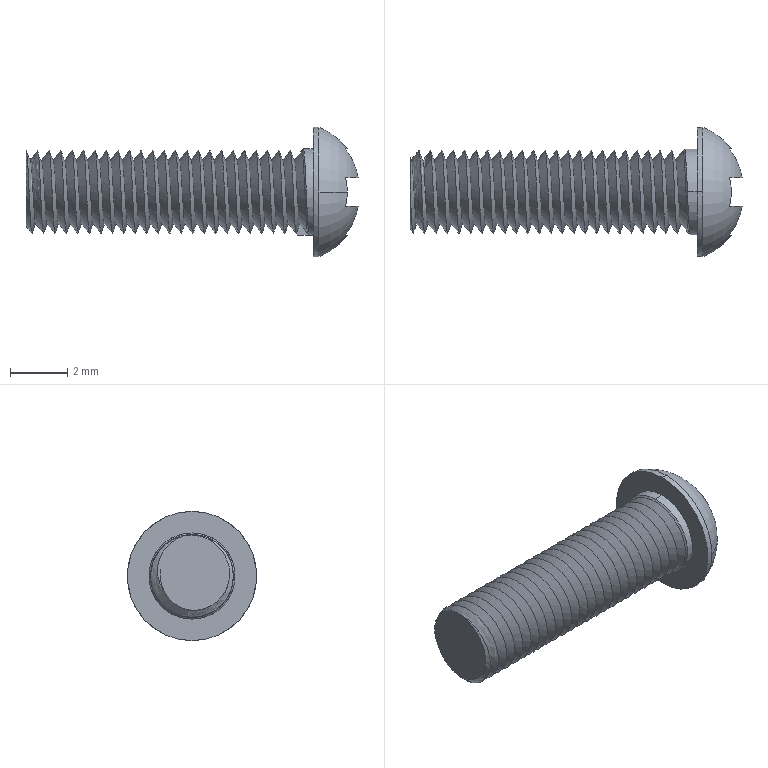Part | SolidWorks | features BaseBody 1 | 1 solid | 25 faces | box 11.56 x 4.5 x 4.5 mm | volume 63.783 mm3 | plane 16 | cylinder 4 | spline 3 | torus 2 | commonest cylinder face diameters 3 x2 4.5 x2